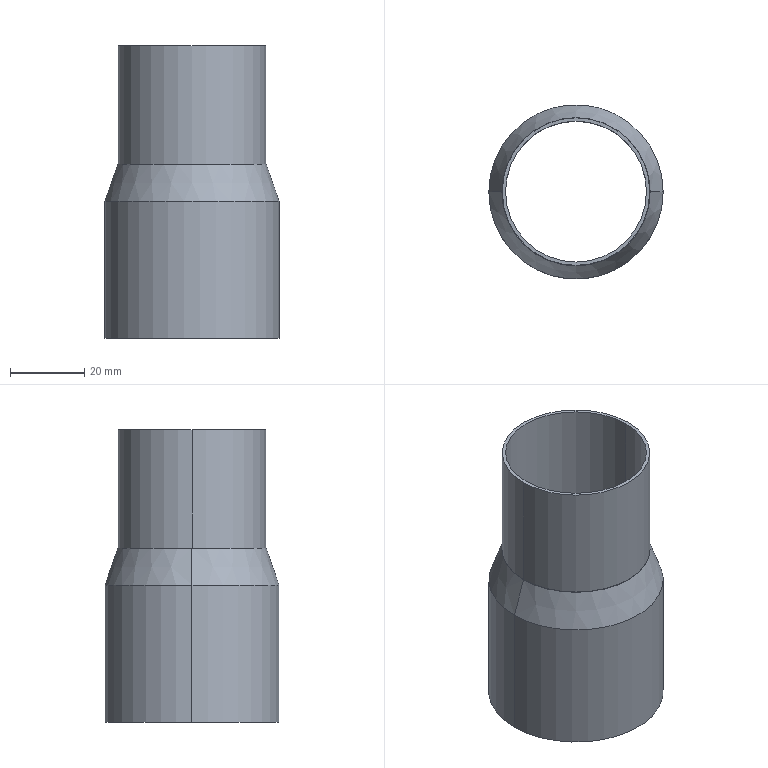Part | SolidWorks | features 3DProfileFeature 2, ICE 2, NetBlend 1, NetBlendCut 1 | 1 solid | 15 faces | box 47 x 47 x 79 mm | volume 10172 mm3 | cylinder 8 | cone 4 | plane 3 | commonest cylinder face diameters 38 x2 39.785 x2 45 x2 47 x2
STEP:
#1=CARTESIAN_POINT('',(-19.,0.,42.));
#2=VERTEX_POINT('',#1);
#3=CARTESIAN_POINT('',(19.,0.,42.));
#4=VERTEX_POINT('',#3);
#5=CARTESIAN_POINT('',(0.,0.,42.));
#6=DIRECTION('',(0.,0.,1.));
#7=DIRECTION('',(1.,0.,0.));
#8=AXIS2_PLACEMENT_3D('',#5,#6,#7);
#9=CIRCLE('',#8,19.);
#10=EDGE_CURVE('',#2,#4,#9,.T.);
#11=ORIENTED_EDGE('',*,*,#10,.T.);
#12=CARTESIAN_POINT('',(19.,0.,10.));
#13=VERTEX_POINT('',#12);
#14=CARTESIAN_POINT('',(19.,0.,42.));
#15=DIRECTION('',(0.,0.,-1.));
#16=VECTOR('',#15,1000.);
#17=LINE('',#14,#16);
#18=EDGE_CURVE('',#4,#13,#17,.T.);
#19=ORIENTED_EDGE('',*,*,#18,.T.);
#20=CARTESIAN_POINT('',(-19.,0.,10.));
#21=VERTEX_POINT('',#20);
#22=CARTESIAN_POINT('',(0.,0.,10.));
#23=DIRECTION('',(0.,0.,-1.));
#24=DIRECTION('',(1.,0.,0.));
#25=AXIS2_PLACEMENT_3D('',#22,#23,#24);
#26=CIRCLE('',#25,19.);
#27=EDGE_CURVE('',#13,#21,#26,.T.);
#28=ORIENTED_EDGE('',*,*,#27,.T.);
#29=CARTESIAN_POINT('',(-19.,0.,42.));
#30=DIRECTION('',(0.,0.,-1.));
#31=VECTOR('',#30,1000.);
#32=LINE('',#29,#31);
#33=EDGE_CURVE('',#2,#21,#32,.T.);
#34=ORIENTED_EDGE('',*,*,#33,.F.);
#35=EDGE_LOOP('',(#11,#19,#28,#34));
#36=FACE_OUTER_BOUND('',#35,.T.);
#37=CARTESIAN_POINT('',(0.,0.,42.));
#38=DIRECTION('',(0.,0.,-1.));
#39=DIRECTION('',(-1.,0.,0.));
#40=AXIS2_PLACEMENT_3D('',#37,#38,#39);
#41=CYLINDRICAL_SURFACE('',#40,19.);
#42=ADVANCED_FACE('',(#36),#41,.F.);
#43=CARTESIAN_POINT('',(19.893,0.,42.));
#44=VERTEX_POINT('',#43);
#45=CARTESIAN_POINT('',(-19.893,0.,42.));
#46=VERTEX_POINT('',#45);
#47=CARTESIAN_POINT('',(0.,0.,42.));
#48=DIRECTION('',(0.,0.,1.));
#49=DIRECTION('',(1.,0.,0.));
#50=AXIS2_PLACEMENT_3D('',#47,#48,#49);
#51=CIRCLE('',#50,19.893);
#52=EDGE_CURVE('',#44,#46,#51,.T.);
#53=ORIENTED_EDGE('',*,*,#52,.F.);
#54=CARTESIAN_POINT('',(19.893,0.,10.));
#55=VERTEX_POINT('',#54);
#56=CARTESIAN_POINT('',(19.893,0.,42.));
#57=DIRECTION('',(0.,0.,-1.));
#58=VECTOR('',#57,1000.);
#59=LINE('',#56,#58);
#60=EDGE_CURVE('',#44,#55,#59,.T.);
#61=ORIENTED_EDGE('',*,*,#60,.T.);
#62=CARTESIAN_POINT('',(-19.893,0.,10.));
#63=VERTEX_POINT('',#62);
#64=CARTESIAN_POINT('',(0.,0.,10.));
#65=DIRECTION('',(0.,0.,1.));
#66=DIRECTION('',(1.,0.,0.));
#67=AXIS2_PLACEMENT_3D('',#64,#65,#66);
#68=CIRCLE('',#67,19.893);
#69=EDGE_CURVE('',#55,#63,#68,.T.);
#70=ORIENTED_EDGE('',*,*,#69,.T.);
#71=CARTESIAN_POINT('',(-19.893,0.,42.));
#72=DIRECTION('',(0.,0.,-1.));
#73=VECTOR('',#72,1000.);
#74=LINE('',#71,#73);
#75=EDGE_CURVE('',#46,#63,#74,.T.);
#76=ORIENTED_EDGE('',*,*,#75,.F.);
#77=EDGE_LOOP('',(#53,#61,#70,#76));
#78=FACE_OUTER_BOUND('',#77,.T.);
#79=CARTESIAN_POINT('',(0.,0.,42.));
#80=DIRECTION('',(0.,0.,-1.));
#81=DIRECTION('',(-1.,0.,0.));
#82=AXIS2_PLACEMENT_3D('',#79,#80,#81);
#83=CYLINDRICAL_SURFACE('',#82,19.893);
#84=ADVANCED_FACE('',(#78),#83,.T.);
#85=CARTESIAN_POINT('',(22.5,0.,-37.));
#86=VERTEX_POINT('',#85);
#87=CARTESIAN_POINT('',(-22.5,0.,-37.));
#88=VERTEX_POINT('',#87);
#89=CARTESIAN_POINT('',(0.,0.,-37.));
#90=DIRECTION('',(0.,0.,-1.));
#91=DIRECTION('',(-1.,0.,0.));
#92=AXIS2_PLACEMENT_3D('',#89,#90,#91);
#93=CIRCLE('',#92,22.5);
#94=EDGE_CURVE('',#86,#88,#93,.T.);
#95=ORIENTED_EDGE('',*,*,#94,.T.);
#96=CARTESIAN_POINT('',(-22.5,0.,0.));
#97=VERTEX_POINT('',#96);
#98=CARTESIAN_POINT('',(-22.5,0.,-37.));
#99=DIRECTION('',(0.,0.,1.));
#100=VECTOR('',#99,1000.);
#101=LINE('',#98,#100);
#102=EDGE_CURVE('',#88,#97,#101,.T.);
#103=ORIENTED_EDGE('',*,*,#102,.T.);
#104=CARTESIAN_POINT('',(22.5,0.,0.));
#105=VERTEX_POINT('',#104);
#106=CARTESIAN_POINT('',(0.,0.,0.));
#107=DIRECTION('',(0.,0.,-1.));
#108=DIRECTION('',(-1.,0.,0.));
#109=AXIS2_PLACEMENT_3D('',#106,#107,#108);
#110=CIRCLE('',#109,22.5);
#111=EDGE_CURVE('',#105,#97,#110,.T.);
#112=ORIENTED_EDGE('',*,*,#111,.F.);
#113=CARTESIAN_POINT('',(22.5,0.,-37.));
#114=DIRECTION('',(0.,0.,1.));
#115=VECTOR('',#114,1000.);
#116=LINE('',#113,#115);
#117=EDGE_CURVE('',#86,#105,#116,.T.);
#118=ORIENTED_EDGE('',*,*,#117,.F.);
#119=EDGE_LOOP('',(#95,#103,#112,#118));
#120=FACE_OUTER_BOUND('',#119,.T.);
#121=CARTESIAN_POINT('',(0.,0.,-37.));
#122=DIRECTION('',(0.,0.,1.));
#123=DIRECTION('',(1.,0.,0.));
#124=AXIS2_PLACEMENT_3D('',#121,#122,#123);
#125=CYLINDRICAL_SURFACE('',#124,22.5);
#126=ADVANCED_FACE('',(#120),#125,.F.);
#127=CARTESIAN_POINT('',(-23.5,0.,-37.));
#128=VERTEX_POINT('',#127);
#129=CARTESIAN_POINT('',(23.5,0.,-37.));
#130=VERTEX_POINT('',#129);
#131=CARTESIAN_POINT('',(0.,0.,-37.));
#132=DIRECTION('',(0.,0.,-1.));
#133=DIRECTION('',(-1.,0.,0.));
#134=AXIS2_PLACEMENT_3D('',#131,#132,#133);
#135=CIRCLE('',#134,23.5);
#136=EDGE_CURVE('',#128,#130,#135,.T.);
#137=ORIENTED_EDGE('',*,*,#136,.F.);
#138=CARTESIAN_POINT('',(-23.5,0.,0.));
#139=VERTEX_POINT('',#138);
#140=CARTESIAN_POINT('',(-23.5,0.,-37.));
#141=DIRECTION('',(0.,0.,1.));
#142=VECTOR('',#141,1000.);
#143=LINE('',#140,#142);
#144=EDGE_CURVE('',#128,#139,#143,.T.);
#145=ORIENTED_EDGE('',*,*,#144,.T.);
#146=CARTESIAN_POINT('',(23.5,0.,0.));
#147=VERTEX_POINT('',#146);
#148=CARTESIAN_POINT('',(0.,0.,0.));
#149=DIRECTION('',(0.,0.,-1.));
#150=DIRECTION('',(-1.,0.,0.));
#151=AXIS2_PLACEMENT_3D('',#148,#149,#150);
#152=CIRCLE('',#151,23.5);
#153=EDGE_CURVE('',#139,#147,#152,.T.);
#154=ORIENTED_EDGE('',*,*,#153,.T.);
#155=CARTESIAN_POINT('',(23.5,0.,-37.));
#156=DIRECTION('',(0.,0.,1.));
#157=VECTOR('',#156,1000.);
#158=LINE('',#155,#157);
#159=EDGE_CURVE('',#130,#147,#158,.T.);
#160=ORIENTED_EDGE('',*,*,#159,.F.);
#161=EDGE_LOOP('',(#137,#145,#154,#160));
#162=FACE_OUTER_BOUND('',#161,.T.);
#163=CARTESIAN_POINT('',(0.,0.,-37.));
#164=DIRECTION('',(0.,0.,1.));
#165=DIRECTION('',(1.,0.,0.));
#166=AXIS2_PLACEMENT_3D('',#163,#164,#165);
#167=CYLINDRICAL_SURFACE('',#166,23.5);
#168=ADVANCED_FACE('',(#162),#167,.T.);
#169=ORIENTED_EDGE('',*,*,#27,.F.);
#170=CARTESIAN_POINT('',(19.,0.,10.));
#171=DIRECTION('',(0.3304,0.,-0.9439));
#172=VECTOR('',#171,1000.);
#173=LINE('',#170,#172);
#174=EDGE_CURVE('',#13,#105,#173,.T.);
#175=ORIENTED_EDGE('',*,*,#174,.T.);
#176=ORIENTED_EDGE('',*,*,#111,.T.);
#177=CARTESIAN_POINT('',(-19.,0.,10.));
#178=DIRECTION('',(-0.3304,0.,-0.9439));
#179=VECTOR('',#178,1000.);
#180=LINE('',#177,#179);
#181=EDGE_CURVE('',#21,#97,#180,.T.);
#182=ORIENTED_EDGE('',*,*,#181,.F.);
#183=EDGE_LOOP('',(#169,#175,#176,#182));
#184=FACE_OUTER_BOUND('',#183,.T.);
#185=CARTESIAN_POINT('',(0.,0.,10.));
#186=DIRECTION('',(0.,0.,-1.));
#187=DIRECTION('',(-1.,0.,0.));
#188=AXIS2_PLACEMENT_3D('',#185,#186,#187);
#189=CONICAL_SURFACE('',#188,19.,0.3367);
#190=ADVANCED_FACE('',(#184),#189,.F.);
#191=CARTESIAN_POINT('',(20.,0.000000029,10.));
#192=VERTEX_POINT('',#191);
#193=CARTESIAN_POINT('',(-20.,0.000000244,10.));
#194=VERTEX_POINT('',#193);
#195=CARTESIAN_POINT('',(0.,0.,10.));
#196=DIRECTION('',(0.,0.,1.));
#197=DIRECTION('',(1.,0.,0.));
#198=AXIS2_PLACEMENT_3D('',#195,#196,#197);
#199=CIRCLE('',#198,20.);
#200=EDGE_CURVE('',#192,#194,#199,.T.);
#201=ORIENTED_EDGE('',*,*,#200,.F.);
#202=CARTESIAN_POINT('',(20.,0.,10.));
#203=DIRECTION('',(0.3304,0.,-0.9439));
#204=VECTOR('',#203,1000.);
#205=LINE('',#202,#204);
#206=EDGE_CURVE('',#192,#147,#205,.T.);
#207=ORIENTED_EDGE('',*,*,#206,.T.);
#208=ORIENTED_EDGE('',*,*,#153,.F.);
#209=CARTESIAN_POINT('',(-20.,0.,10.));
#210=DIRECTION('',(-0.3304,0.,-0.9439));
#211=VECTOR('',#210,1000.);
#212=LINE('',#209,#211);
#213=EDGE_CURVE('',#194,#139,#212,.T.);
#214=ORIENTED_EDGE('',*,*,#213,.F.);
#215=EDGE_LOOP('',(#201,#207,#208,#214));
#216=FACE_OUTER_BOUND('',#215,.T.);
#217=CARTESIAN_POINT('',(0.,0.,10.));
#218=DIRECTION('',(0.,0.,-1.));
#219=DIRECTION('',(-1.,0.,0.));
#220=AXIS2_PLACEMENT_3D('',#217,#218,#219);
#221=CONICAL_SURFACE('',#220,20.,0.3367);
#222=ADVANCED_FACE('',(#216),#221,.T.);
#223=CARTESIAN_POINT('',(0.,0.,10.));
#224=DIRECTION('',(0.,0.,1.));
#225=DIRECTION('',(1.,0.,0.));
#226=AXIS2_PLACEMENT_3D('',#223,#224,#225);
#227=CIRCLE('',#226,20.);
#228=EDGE_CURVE('',#194,#192,#227,.T.);
#229=ORIENTED_EDGE('',*,*,#228,.T.);
#230=ORIENTED_EDGE('',*,*,#200,.T.);
#231=EDGE_LOOP('',(#229,#230));
#232=FACE_OUTER_BOUND('',#231,.T.);
#233=CARTESIAN_POINT('',(0.,0.,10.));
#234=DIRECTION('',(0.,0.,1.));
#235=DIRECTION('',(1.,0.,0.));
#236=AXIS2_PLACEMENT_3D('',#233,#234,#235);
#237=CIRCLE('',#236,19.893);
#238=EDGE_CURVE('',#63,#55,#237,.T.);
#239=ORIENTED_EDGE('',*,*,#238,.F.);
#240=ORIENTED_EDGE('',*,*,#69,.F.);
#241=EDGE_LOOP('',(#239,#240));
#242=FACE_BOUND('',#241,.T.);
#243=CARTESIAN_POINT('',(0.,0.,10.));
#244=DIRECTION('',(0.,0.,1.));
#245=DIRECTION('',(1.,0.,0.));
#246=AXIS2_PLACEMENT_3D('',#243,#244,#245);
#247=PLANE('',#246);
#248=ADVANCED_FACE('',(#232,#242),#247,.T.);
#249=ORIENTED_EDGE('',*,*,#206,.F.);
#250=ORIENTED_EDGE('',*,*,#228,.F.);
#251=ORIENTED_EDGE('',*,*,#213,.T.);
#252=CARTESIAN_POINT('',(0.,0.,0.));
#253=DIRECTION('',(0.,0.,-1.));
#254=DIRECTION('',(-1.,0.,0.));
#255=AXIS2_PLACEMENT_3D('',#252,#253,#254);
#256=CIRCLE('',#255,23.5);
#257=EDGE_CURVE('',#147,#139,#256,.T.);
#258=ORIENTED_EDGE('',*,*,#257,.F.);
#259=EDGE_LOOP('',(#249,#250,#251,#258));
#260=FACE_OUTER_BOUND('',#259,.T.);
#261=CARTESIAN_POINT('',(0.,0.,10.));
#262=DIRECTION('',(0.,0.,-1.));
#263=DIRECTION('',(-1.,0.,0.));
#264=AXIS2_PLACEMENT_3D('',#261,#262,#263);
#265=CONICAL_SURFACE('',#264,20.,0.3367);
#266=ADVANCED_FACE('',(#260),#265,.T.);
#267=ORIENTED_EDGE('',*,*,#174,.F.);
#268=CARTESIAN_POINT('',(0.,0.,10.));
#269=DIRECTION('',(0.,0.,-1.));
#270=DIRECTION('',(1.,0.,0.));
#271=AXIS2_PLACEMENT_3D('',#268,#269,#270);
#272=CIRCLE('',#271,19.);
#273=EDGE_CURVE('',#21,#13,#272,.T.);
#274=ORIENTED_EDGE('',*,*,#273,.F.);
#275=ORIENTED_EDGE('',*,*,#181,.T.);
#276=CARTESIAN_POINT('',(0.,0.,0.));
#277=DIRECTION('',(0.,0.,-1.));
#278=DIRECTION('',(-1.,0.,0.));
#279=AXIS2_PLACEMENT_3D('',#276,#277,#278);
#280=CIRCLE('',#279,22.5);
#281=EDGE_CURVE('',#97,#105,#280,.T.);
#282=ORIENTED_EDGE('',*,*,#281,.T.);
#283=EDGE_LOOP('',(#267,#274,#275,#282));
#284=FACE_OUTER_BOUND('',#283,.T.);
#285=CARTESIAN_POINT('',(0.,0.,10.));
#286=DIRECTION('',(0.,0.,-1.));
#287=DIRECTION('',(-1.,0.,0.));
#288=AXIS2_PLACEMENT_3D('',#285,#286,#287);
#289=CONICAL_SURFACE('',#288,19.,0.3367);
#290=ADVANCED_FACE('',(#284),#289,.F.);
#291=CARTESIAN_POINT('',(0.,0.,-37.));
#292=DIRECTION('',(0.,0.,-1.));
#293=DIRECTION('',(-1.,0.,0.));
#294=AXIS2_PLACEMENT_3D('',#291,#292,#293);
#295=CIRCLE('',#294,23.5);
#296=EDGE_CURVE('',#130,#128,#295,.T.);
#297=ORIENTED_EDGE('',*,*,#296,.T.);
#298=ORIENTED_EDGE('',*,*,#136,.T.);
#299=EDGE_LOOP('',(#297,#298));
#300=FACE_OUTER_BOUND('',#299,.T.);
#301=ORIENTED_EDGE('',*,*,#94,.F.);
#302=CARTESIAN_POINT('',(0.,0.,-37.));
#303=DIRECTION('',(0.,0.,-1.));
#304=DIRECTION('',(-1.,0.,0.));
#305=AXIS2_PLACEMENT_3D('',#302,#303,#304);
#306=CIRCLE('',#305,22.5);
#307=EDGE_CURVE('',#88,#86,#306,.T.);
#308=ORIENTED_EDGE('',*,*,#307,.F.);
#309=EDGE_LOOP('',(#301,#308));
#310=FACE_BOUND('',#309,.T.);
#311=CARTESIAN_POINT('',(0.,0.,-37.));
#312=DIRECTION('',(0.,0.,-1.));
#313=DIRECTION('',(-1.,0.,0.));
#314=AXIS2_PLACEMENT_3D('',#311,#312,#313);
#315=PLANE('',#314);
#316=ADVANCED_FACE('',(#300,#310),#315,.T.);
#317=ORIENTED_EDGE('',*,*,#144,.F.);
#318=ORIENTED_EDGE('',*,*,#296,.F.);
#319=ORIENTED_EDGE('',*,*,#159,.T.);
#320=ORIENTED_EDGE('',*,*,#257,.T.);
#321=EDGE_LOOP('',(#317,#318,#319,#320));
#322=FACE_OUTER_BOUND('',#321,.T.);
#323=CARTESIAN_POINT('',(0.,0.,-37.));
#324=DIRECTION('',(0.,0.,1.));
#325=DIRECTION('',(1.,0.,0.));
#326=AXIS2_PLACEMENT_3D('',#323,#324,#325);
#327=CYLINDRICAL_SURFACE('',#326,23.5);
#328=ADVANCED_FACE('',(#322),#327,.T.);
#329=ORIENTED_EDGE('',*,*,#102,.F.);
#330=ORIENTED_EDGE('',*,*,#307,.T.);
#331=ORIENTED_EDGE('',*,*,#117,.T.);
#332=ORIENTED_EDGE('',*,*,#281,.F.);
#333=EDGE_LOOP('',(#329,#330,#331,#332));
#334=FACE_OUTER_BOUND('',#333,.T.);
#335=CARTESIAN_POINT('',(0.,0.,-37.));
#336=DIRECTION('',(0.,0.,1.));
#337=DIRECTION('',(1.,0.,0.));
#338=AXIS2_PLACEMENT_3D('',#335,#336,#337);
#339=CYLINDRICAL_SURFACE('',#338,22.5);
#340=ADVANCED_FACE('',(#334),#339,.F.);
#341=CARTESIAN_POINT('',(0.,0.,42.));
#342=DIRECTION('',(0.,0.,1.));
#343=DIRECTION('',(1.,0.,0.));
#344=AXIS2_PLACEMENT_3D('',#341,#342,#343);
#345=CIRCLE('',#344,19.893);
#346=EDGE_CURVE('',#46,#44,#345,.T.);
#347=ORIENTED_EDGE('',*,*,#346,.T.);
#348=ORIENTED_EDGE('',*,*,#52,.T.);
#349=EDGE_LOOP('',(#347,#348));
#350=FACE_OUTER_BOUND('',#349,.T.);
#351=ORIENTED_EDGE('',*,*,#10,.F.);
#352=CARTESIAN_POINT('',(0.,0.,42.));
#353=DIRECTION('',(0.,0.,1.));
#354=DIRECTION('',(1.,0.,0.));
#355=AXIS2_PLACEMENT_3D('',#352,#353,#354);
#356=CIRCLE('',#355,19.);
#357=EDGE_CURVE('',#4,#2,#356,.T.);
#358=ORIENTED_EDGE('',*,*,#357,.F.);
#359=EDGE_LOOP('',(#351,#358));
#360=FACE_BOUND('',#359,.T.);
#361=CARTESIAN_POINT('',(0.,0.,42.));
#362=DIRECTION('',(0.,0.,1.));
#363=DIRECTION('',(1.,0.,0.));
#364=AXIS2_PLACEMENT_3D('',#361,#362,#363);
#365=PLANE('',#364);
#366=ADVANCED_FACE('',(#350,#360),#365,.T.);
#367=ORIENTED_EDGE('',*,*,#60,.F.);
#368=ORIENTED_EDGE('',*,*,#346,.F.);
#369=ORIENTED_EDGE('',*,*,#75,.T.);
#370=ORIENTED_EDGE('',*,*,#238,.T.);
#371=EDGE_LOOP('',(#367,#368,#369,#370));
#372=FACE_OUTER_BOUND('',#371,.T.);
#373=CARTESIAN_POINT('',(0.,0.,42.));
#374=DIRECTION('',(0.,0.,-1.));
#375=DIRECTION('',(-1.,0.,0.));
#376=AXIS2_PLACEMENT_3D('',#373,#374,#375);
#377=CYLINDRICAL_SURFACE('',#376,19.893);
#378=ADVANCED_FACE('',(#372),#377,.T.);
#379=ORIENTED_EDGE('',*,*,#18,.F.);
#380=ORIENTED_EDGE('',*,*,#357,.T.);
#381=ORIENTED_EDGE('',*,*,#33,.T.);
#382=ORIENTED_EDGE('',*,*,#273,.T.);
#383=EDGE_LOOP('',(#379,#380,#381,#382));
#384=FACE_OUTER_BOUND('',#383,.T.);
#385=CARTESIAN_POINT('',(0.,0.,42.));
#386=DIRECTION('',(0.,0.,-1.));
#387=DIRECTION('',(-1.,0.,0.));
#388=AXIS2_PLACEMENT_3D('',#385,#386,#387);
#389=CYLINDRICAL_SURFACE('',#388,19.);
#390=ADVANCED_FACE('',(#384),#389,.F.);
#391=CLOSED_SHELL('',(#42,#84,#126,#168,#190,#222,#248,#266,#290,#316,#328,#340,#366,#378,#390));
#392=MANIFOLD_SOLID_BREP('',#391);
#393=CARTESIAN_POINT('',(0.,0.,0.));
#394=DIRECTION('',(0.,0.,1.));
#395=DIRECTION('',(1.,0.,0.));
#396=AXIS2_PLACEMENT_3D('',#393,#394,#395);
#397=(LENGTH_UNIT()NAMED_UNIT(*)SI_UNIT(.MILLI.,.METRE.));
#398=UNCERTAINTY_MEASURE_WITH_UNIT(LENGTH_MEASURE(0.00001),#397,'','');
#399=(NAMED_UNIT(*)PLANE_ANGLE_UNIT()SI_UNIT($,.RADIAN.));
#400=(NAMED_UNIT(*)SI_UNIT($,.STERADIAN.)SOLID_ANGLE_UNIT());
#401=(GEOMETRIC_REPRESENTATION_CONTEXT(3)GLOBAL_UNCERTAINTY_ASSIGNED_CONTEXT((#398))GLOBAL_UNIT_ASSIGNED_CONTEXT((#397,#399,#400))REPRESENTATION_CONTEXT('',''));
#402=ADVANCED_BREP_SHAPE_REPRESENTATION('',(#392,#396),#401);